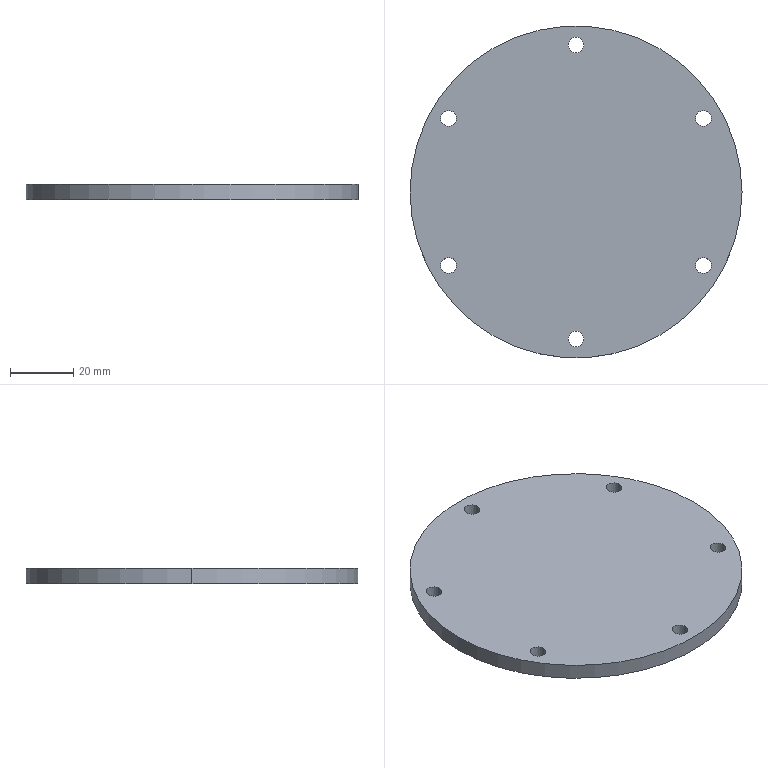Part | STEP file | smoke vent cover plate | 1 solid | 16 faces | box 105 x 105 x 5 mm | volume 42706 mm3 | cylinder 14 | plane 2 | commonest cylinder face diameters 5 x12 105 x2
STEP:
#1=CARTESIAN_POINT('',(0.,0.,0.));
#2=DIRECTION('',(0.,0.,1.));
#3=DIRECTION('',(1.,0.,0.));
#4=AXIS2_PLACEMENT_3D('',#1,#2,#3);
#5=CARTESIAN_POINT('',(-42.77,23.25,5.));
#6=VERTEX_POINT('',#5);
#7=CARTESIAN_POINT('',(-42.77,23.25,0.));
#8=VERTEX_POINT('',#7);
#9=CARTESIAN_POINT('',(-42.77,23.25,5.));
#10=DIRECTION('',(0.,0.,-1.));
#11=VECTOR('',#10,1.);
#12=LINE('',#9,#11);
#13=CARTESIAN_POINT('',(-40.27,23.25,5.));
#14=DIRECTION('',(0.,0.,-1.));
#15=DIRECTION('',(-1.,0.,0.));
#16=AXIS2_PLACEMENT_3D('',#13,#14,#15);
#17=CYLINDRICAL_SURFACE('',#16,2.5);
#18=CARTESIAN_POINT('',(6.283,0.));
#19=DIRECTION('',(0.,1.));
#20=VECTOR('',#19,1.);
#21=LINE('',#18,#20);
#22=(GEOMETRIC_REPRESENTATION_CONTEXT(2)PARAMETRIC_REPRESENTATION_CONTEXT()REPRESENTATION_CONTEXT('',''));
#23=DEFINITIONAL_REPRESENTATION('',(#21),#22);
#24=PCURVE('',#17,#23);
#25=CARTESIAN_POINT('',(-40.27,23.25,5.));
#26=DIRECTION('',(0.,0.,-1.));
#27=DIRECTION('',(-1.,0.,0.));
#28=AXIS2_PLACEMENT_3D('',#25,#26,#27);
#29=CYLINDRICAL_SURFACE('',#28,2.5);
#30=CARTESIAN_POINT('',(0.,0.));
#31=DIRECTION('',(0.,1.));
#32=VECTOR('',#31,1.);
#33=LINE('',#30,#32);
#34=(GEOMETRIC_REPRESENTATION_CONTEXT(2)PARAMETRIC_REPRESENTATION_CONTEXT()REPRESENTATION_CONTEXT('',''));
#35=DEFINITIONAL_REPRESENTATION('',(#33),#34);
#36=PCURVE('',#29,#35);
#37=SURFACE_CURVE('',#12,(#24,#36),.PCURVE_S1.);
#38=EDGE_CURVE('',#6,#8,#37,.T.);
#39=ORIENTED_EDGE('',*,*,#38,.T.);
#40=CARTESIAN_POINT('',(-37.77,23.25,0.));
#41=VERTEX_POINT('',#40);
#42=CARTESIAN_POINT('',(-40.27,23.25,0.));
#43=DIRECTION('',(0.,0.,1.));
#44=DIRECTION('',(1.,0.,0.));
#45=AXIS2_PLACEMENT_3D('',#42,#43,#44);
#46=CIRCLE('',#45,2.5);
#47=CARTESIAN_POINT('',(9.425,5.));
#48=DIRECTION('',(-1.,0.));
#49=VECTOR('',#48,1.);
#50=LINE('',#47,#49);
#51=(GEOMETRIC_REPRESENTATION_CONTEXT(2)PARAMETRIC_REPRESENTATION_CONTEXT()REPRESENTATION_CONTEXT('',''));
#52=DEFINITIONAL_REPRESENTATION('',(#50),#51);
#53=PCURVE('',#17,#52);
#54=CARTESIAN_POINT('',(0.,0.,0.));
#55=DIRECTION('',(0.,0.,1.));
#56=DIRECTION('',(1.,0.,0.));
#57=AXIS2_PLACEMENT_3D('',#54,#55,#56);
#58=PLANE('',#57);
#59=CARTESIAN_POINT('',(-40.27,23.25));
#60=DIRECTION('',(1.,0.));
#61=AXIS2_PLACEMENT_2D('',#59,#60);
#62=CIRCLE('',#61,2.5);
#63=(GEOMETRIC_REPRESENTATION_CONTEXT(2)PARAMETRIC_REPRESENTATION_CONTEXT()REPRESENTATION_CONTEXT('',''));
#64=DEFINITIONAL_REPRESENTATION('',(#62),#63);
#65=PCURVE('',#58,#64);
#66=SURFACE_CURVE('',#46,(#53,#65),.PCURVE_S1.);
#67=EDGE_CURVE('',#8,#41,#66,.T.);
#68=ORIENTED_EDGE('',*,*,#67,.T.);
#69=CARTESIAN_POINT('',(-37.77,23.25,5.));
#70=VERTEX_POINT('',#69);
#71=CARTESIAN_POINT('',(-37.77,23.25,5.));
#72=DIRECTION('',(0.,0.,-1.));
#73=VECTOR('',#72,1.);
#74=LINE('',#71,#73);
#75=CARTESIAN_POINT('',(3.142,0.));
#76=DIRECTION('',(0.,1.));
#77=VECTOR('',#76,1.);
#78=LINE('',#75,#77);
#79=(GEOMETRIC_REPRESENTATION_CONTEXT(2)PARAMETRIC_REPRESENTATION_CONTEXT()REPRESENTATION_CONTEXT('',''));
#80=DEFINITIONAL_REPRESENTATION('',(#78),#79);
#81=PCURVE('',#17,#80);
#82=CARTESIAN_POINT('',(3.142,0.));
#83=DIRECTION('',(0.,1.));
#84=VECTOR('',#83,1.);
#85=LINE('',#82,#84);
#86=(GEOMETRIC_REPRESENTATION_CONTEXT(2)PARAMETRIC_REPRESENTATION_CONTEXT()REPRESENTATION_CONTEXT('',''));
#87=DEFINITIONAL_REPRESENTATION('',(#85),#86);
#88=PCURVE('',#29,#87);
#89=SURFACE_CURVE('',#74,(#81,#88),.PCURVE_S1.);
#90=EDGE_CURVE('',#70,#41,#89,.T.);
#91=ORIENTED_EDGE('',*,*,#90,.F.);
#92=CARTESIAN_POINT('',(-40.27,23.25,5.));
#93=DIRECTION('',(0.,0.,1.));
#94=DIRECTION('',(1.,0.,0.));
#95=AXIS2_PLACEMENT_3D('',#92,#93,#94);
#96=CIRCLE('',#95,2.5);
#97=CARTESIAN_POINT('',(9.425,0.));
#98=DIRECTION('',(-1.,0.));
#99=VECTOR('',#98,1.);
#100=LINE('',#97,#99);
#101=(GEOMETRIC_REPRESENTATION_CONTEXT(2)PARAMETRIC_REPRESENTATION_CONTEXT()REPRESENTATION_CONTEXT('',''));
#102=DEFINITIONAL_REPRESENTATION('',(#100),#101);
#103=PCURVE('',#17,#102);
#104=CARTESIAN_POINT('',(0.,0.,5.));
#105=DIRECTION('',(0.,0.,1.));
#106=DIRECTION('',(1.,0.,0.));
#107=AXIS2_PLACEMENT_3D('',#104,#105,#106);
#108=PLANE('',#107);
#109=CARTESIAN_POINT('',(-40.27,23.25));
#110=DIRECTION('',(1.,0.));
#111=AXIS2_PLACEMENT_2D('',#109,#110);
#112=CIRCLE('',#111,2.5);
#113=(GEOMETRIC_REPRESENTATION_CONTEXT(2)PARAMETRIC_REPRESENTATION_CONTEXT()REPRESENTATION_CONTEXT('',''));
#114=DEFINITIONAL_REPRESENTATION('',(#112),#113);
#115=PCURVE('',#108,#114);
#116=SURFACE_CURVE('',#96,(#103,#115),.PCURVE_S1.);
#117=EDGE_CURVE('',#6,#70,#116,.T.);
#118=ORIENTED_EDGE('',*,*,#117,.F.);
#119=EDGE_LOOP('',(#39,#68,#91,#118));
#120=FACE_BOUND('',#119,.F.);
#121=ADVANCED_FACE('',(#120),#17,.F.);
#122=CARTESIAN_POINT('',(-42.77,-23.25,5.));
#123=VERTEX_POINT('',#122);
#124=CARTESIAN_POINT('',(-42.77,-23.25,0.));
#125=VERTEX_POINT('',#124);
#126=CARTESIAN_POINT('',(-42.77,-23.25,5.));
#127=DIRECTION('',(0.,0.,-1.));
#128=VECTOR('',#127,1.);
#129=LINE('',#126,#128);
#130=CARTESIAN_POINT('',(-40.27,-23.25,5.));
#131=DIRECTION('',(0.,0.,-1.));
#132=DIRECTION('',(-1.,0.,0.));
#133=AXIS2_PLACEMENT_3D('',#130,#131,#132);
#134=CYLINDRICAL_SURFACE('',#133,2.5);
#135=CARTESIAN_POINT('',(6.283,0.));
#136=DIRECTION('',(0.,1.));
#137=VECTOR('',#136,1.);
#138=LINE('',#135,#137);
#139=(GEOMETRIC_REPRESENTATION_CONTEXT(2)PARAMETRIC_REPRESENTATION_CONTEXT()REPRESENTATION_CONTEXT('',''));
#140=DEFINITIONAL_REPRESENTATION('',(#138),#139);
#141=PCURVE('',#134,#140);
#142=CARTESIAN_POINT('',(-40.27,-23.25,5.));
#143=DIRECTION('',(0.,0.,-1.));
#144=DIRECTION('',(-1.,0.,0.));
#145=AXIS2_PLACEMENT_3D('',#142,#143,#144);
#146=CYLINDRICAL_SURFACE('',#145,2.5);
#147=CARTESIAN_POINT('',(0.,0.));
#148=DIRECTION('',(0.,1.));
#149=VECTOR('',#148,1.);
#150=LINE('',#147,#149);
#151=(GEOMETRIC_REPRESENTATION_CONTEXT(2)PARAMETRIC_REPRESENTATION_CONTEXT()REPRESENTATION_CONTEXT('',''));
#152=DEFINITIONAL_REPRESENTATION('',(#150),#151);
#153=PCURVE('',#146,#152);
#154=SURFACE_CURVE('',#129,(#141,#153),.PCURVE_S1.);
#155=EDGE_CURVE('',#123,#125,#154,.T.);
#156=ORIENTED_EDGE('',*,*,#155,.T.);
#157=CARTESIAN_POINT('',(-37.77,-23.25,0.));
#158=VERTEX_POINT('',#157);
#159=CARTESIAN_POINT('',(-40.27,-23.25,0.));
#160=DIRECTION('',(0.,0.,1.));
#161=DIRECTION('',(1.,0.,0.));
#162=AXIS2_PLACEMENT_3D('',#159,#160,#161);
#163=CIRCLE('',#162,2.5);
#164=CARTESIAN_POINT('',(9.425,5.));
#165=DIRECTION('',(-1.,0.));
#166=VECTOR('',#165,1.);
#167=LINE('',#164,#166);
#168=(GEOMETRIC_REPRESENTATION_CONTEXT(2)PARAMETRIC_REPRESENTATION_CONTEXT()REPRESENTATION_CONTEXT('',''));
#169=DEFINITIONAL_REPRESENTATION('',(#167),#168);
#170=PCURVE('',#134,#169);
#171=CARTESIAN_POINT('',(-40.27,-23.25));
#172=DIRECTION('',(1.,0.));
#173=AXIS2_PLACEMENT_2D('',#171,#172);
#174=CIRCLE('',#173,2.5);
#175=(GEOMETRIC_REPRESENTATION_CONTEXT(2)PARAMETRIC_REPRESENTATION_CONTEXT()REPRESENTATION_CONTEXT('',''));
#176=DEFINITIONAL_REPRESENTATION('',(#174),#175);
#177=PCURVE('',#58,#176);
#178=SURFACE_CURVE('',#163,(#170,#177),.PCURVE_S1.);
#179=EDGE_CURVE('',#125,#158,#178,.T.);
#180=ORIENTED_EDGE('',*,*,#179,.T.);
#181=CARTESIAN_POINT('',(-37.77,-23.25,5.));
#182=VERTEX_POINT('',#181);
#183=CARTESIAN_POINT('',(-37.77,-23.25,5.));
#184=DIRECTION('',(0.,0.,-1.));
#185=VECTOR('',#184,1.);
#186=LINE('',#183,#185);
#187=CARTESIAN_POINT('',(3.142,0.));
#188=DIRECTION('',(0.,1.));
#189=VECTOR('',#188,1.);
#190=LINE('',#187,#189);
#191=(GEOMETRIC_REPRESENTATION_CONTEXT(2)PARAMETRIC_REPRESENTATION_CONTEXT()REPRESENTATION_CONTEXT('',''));
#192=DEFINITIONAL_REPRESENTATION('',(#190),#191);
#193=PCURVE('',#134,#192);
#194=CARTESIAN_POINT('',(3.142,0.));
#195=DIRECTION('',(0.,1.));
#196=VECTOR('',#195,1.);
#197=LINE('',#194,#196);
#198=(GEOMETRIC_REPRESENTATION_CONTEXT(2)PARAMETRIC_REPRESENTATION_CONTEXT()REPRESENTATION_CONTEXT('',''));
#199=DEFINITIONAL_REPRESENTATION('',(#197),#198);
#200=PCURVE('',#146,#199);
#201=SURFACE_CURVE('',#186,(#193,#200),.PCURVE_S1.);
#202=EDGE_CURVE('',#182,#158,#201,.T.);
#203=ORIENTED_EDGE('',*,*,#202,.F.);
#204=CARTESIAN_POINT('',(-40.27,-23.25,5.));
#205=DIRECTION('',(0.,0.,1.));
#206=DIRECTION('',(1.,0.,0.));
#207=AXIS2_PLACEMENT_3D('',#204,#205,#206);
#208=CIRCLE('',#207,2.5);
#209=CARTESIAN_POINT('',(9.425,0.));
#210=DIRECTION('',(-1.,0.));
#211=VECTOR('',#210,1.);
#212=LINE('',#209,#211);
#213=(GEOMETRIC_REPRESENTATION_CONTEXT(2)PARAMETRIC_REPRESENTATION_CONTEXT()REPRESENTATION_CONTEXT('',''));
#214=DEFINITIONAL_REPRESENTATION('',(#212),#213);
#215=PCURVE('',#134,#214);
#216=CARTESIAN_POINT('',(-40.27,-23.25));
#217=DIRECTION('',(1.,0.));
#218=AXIS2_PLACEMENT_2D('',#216,#217);
#219=CIRCLE('',#218,2.5);
#220=(GEOMETRIC_REPRESENTATION_CONTEXT(2)PARAMETRIC_REPRESENTATION_CONTEXT()REPRESENTATION_CONTEXT('',''));
#221=DEFINITIONAL_REPRESENTATION('',(#219),#220);
#222=PCURVE('',#108,#221);
#223=SURFACE_CURVE('',#208,(#215,#222),.PCURVE_S1.);
#224=EDGE_CURVE('',#123,#182,#223,.T.);
#225=ORIENTED_EDGE('',*,*,#224,.F.);
#226=EDGE_LOOP('',(#156,#180,#203,#225));
#227=FACE_BOUND('',#226,.F.);
#228=ADVANCED_FACE('',(#227),#134,.F.);
#229=CARTESIAN_POINT('',(-2.5,-46.5,5.));
#230=VERTEX_POINT('',#229);
#231=CARTESIAN_POINT('',(-2.5,-46.5,0.));
#232=VERTEX_POINT('',#231);
#233=CARTESIAN_POINT('',(-2.5,-46.5,5.));
#234=DIRECTION('',(0.,0.,-1.));
#235=VECTOR('',#234,1.);
#236=LINE('',#233,#235);
#237=CARTESIAN_POINT('',(0.,-46.5,5.));
#238=DIRECTION('',(0.,0.,-1.));
#239=DIRECTION('',(-1.,0.,0.));
#240=AXIS2_PLACEMENT_3D('',#237,#238,#239);
#241=CYLINDRICAL_SURFACE('',#240,2.5);
#242=CARTESIAN_POINT('',(6.283,0.));
#243=DIRECTION('',(0.,1.));
#244=VECTOR('',#243,1.);
#245=LINE('',#242,#244);
#246=(GEOMETRIC_REPRESENTATION_CONTEXT(2)PARAMETRIC_REPRESENTATION_CONTEXT()REPRESENTATION_CONTEXT('',''));
#247=DEFINITIONAL_REPRESENTATION('',(#245),#246);
#248=PCURVE('',#241,#247);
#249=CARTESIAN_POINT('',(0.,-46.5,5.));
#250=DIRECTION('',(0.,0.,-1.));
#251=DIRECTION('',(-1.,0.,0.));
#252=AXIS2_PLACEMENT_3D('',#249,#250,#251);
#253=CYLINDRICAL_SURFACE('',#252,2.5);
#254=CARTESIAN_POINT('',(0.,0.));
#255=DIRECTION('',(0.,1.));
#256=VECTOR('',#255,1.);
#257=LINE('',#254,#256);
#258=(GEOMETRIC_REPRESENTATION_CONTEXT(2)PARAMETRIC_REPRESENTATION_CONTEXT()REPRESENTATION_CONTEXT('',''));
#259=DEFINITIONAL_REPRESENTATION('',(#257),#258);
#260=PCURVE('',#253,#259);
#261=SURFACE_CURVE('',#236,(#248,#260),.PCURVE_S1.);
#262=EDGE_CURVE('',#230,#232,#261,.T.);
#263=ORIENTED_EDGE('',*,*,#262,.T.);
#264=CARTESIAN_POINT('',(2.5,-46.5,0.));
#265=VERTEX_POINT('',#264);
#266=CARTESIAN_POINT('',(0.,-46.5,0.));
#267=DIRECTION('',(0.,0.,1.));
#268=DIRECTION('',(1.,0.,0.));
#269=AXIS2_PLACEMENT_3D('',#266,#267,#268);
#270=CIRCLE('',#269,2.5);
#271=CARTESIAN_POINT('',(9.425,5.));
#272=DIRECTION('',(-1.,0.));
#273=VECTOR('',#272,1.);
#274=LINE('',#271,#273);
#275=(GEOMETRIC_REPRESENTATION_CONTEXT(2)PARAMETRIC_REPRESENTATION_CONTEXT()REPRESENTATION_CONTEXT('',''));
#276=DEFINITIONAL_REPRESENTATION('',(#274),#275);
#277=PCURVE('',#241,#276);
#278=CARTESIAN_POINT('',(0.,-46.5));
#279=DIRECTION('',(1.,0.));
#280=AXIS2_PLACEMENT_2D('',#278,#279);
#281=CIRCLE('',#280,2.5);
#282=(GEOMETRIC_REPRESENTATION_CONTEXT(2)PARAMETRIC_REPRESENTATION_CONTEXT()REPRESENTATION_CONTEXT('',''));
#283=DEFINITIONAL_REPRESENTATION('',(#281),#282);
#284=PCURVE('',#58,#283);
#285=SURFACE_CURVE('',#270,(#277,#284),.PCURVE_S1.);
#286=EDGE_CURVE('',#232,#265,#285,.T.);
#287=ORIENTED_EDGE('',*,*,#286,.T.);
#288=CARTESIAN_POINT('',(2.5,-46.5,5.));
#289=VERTEX_POINT('',#288);
#290=CARTESIAN_POINT('',(2.5,-46.5,5.));
#291=DIRECTION('',(0.,0.,-1.));
#292=VECTOR('',#291,1.);
#293=LINE('',#290,#292);
#294=CARTESIAN_POINT('',(3.142,0.));
#295=DIRECTION('',(0.,1.));
#296=VECTOR('',#295,1.);
#297=LINE('',#294,#296);
#298=(GEOMETRIC_REPRESENTATION_CONTEXT(2)PARAMETRIC_REPRESENTATION_CONTEXT()REPRESENTATION_CONTEXT('',''));
#299=DEFINITIONAL_REPRESENTATION('',(#297),#298);
#300=PCURVE('',#241,#299);
#301=CARTESIAN_POINT('',(3.142,0.));
#302=DIRECTION('',(0.,1.));
#303=VECTOR('',#302,1.);
#304=LINE('',#301,#303);
#305=(GEOMETRIC_REPRESENTATION_CONTEXT(2)PARAMETRIC_REPRESENTATION_CONTEXT()REPRESENTATION_CONTEXT('',''));
#306=DEFINITIONAL_REPRESENTATION('',(#304),#305);
#307=PCURVE('',#253,#306);
#308=SURFACE_CURVE('',#293,(#300,#307),.PCURVE_S1.);
#309=EDGE_CURVE('',#289,#265,#308,.T.);
#310=ORIENTED_EDGE('',*,*,#309,.F.);
#311=CARTESIAN_POINT('',(0.,-46.5,5.));
#312=DIRECTION('',(0.,0.,1.));
#313=DIRECTION('',(1.,0.,0.));
#314=AXIS2_PLACEMENT_3D('',#311,#312,#313);
#315=CIRCLE('',#314,2.5);
#316=CARTESIAN_POINT('',(9.425,0.));
#317=DIRECTION('',(-1.,0.));
#318=VECTOR('',#317,1.);
#319=LINE('',#316,#318);
#320=(GEOMETRIC_REPRESENTATION_CONTEXT(2)PARAMETRIC_REPRESENTATION_CONTEXT()REPRESENTATION_CONTEXT('',''));
#321=DEFINITIONAL_REPRESENTATION('',(#319),#320);
#322=PCURVE('',#241,#321);
#323=CARTESIAN_POINT('',(0.,-46.5));
#324=DIRECTION('',(1.,0.));
#325=AXIS2_PLACEMENT_2D('',#323,#324);
#326=CIRCLE('',#325,2.5);
#327=(GEOMETRIC_REPRESENTATION_CONTEXT(2)PARAMETRIC_REPRESENTATION_CONTEXT()REPRESENTATION_CONTEXT('',''));
#328=DEFINITIONAL_REPRESENTATION('',(#326),#327);
#329=PCURVE('',#108,#328);
#330=SURFACE_CURVE('',#315,(#322,#329),.PCURVE_S1.);
#331=EDGE_CURVE('',#230,#289,#330,.T.);
#332=ORIENTED_EDGE('',*,*,#331,.F.);
#333=EDGE_LOOP('',(#263,#287,#310,#332));
#334=FACE_BOUND('',#333,.F.);
#335=ADVANCED_FACE('',(#334),#241,.F.);
#336=CARTESIAN_POINT('',(37.77,-23.25,5.));
#337=VERTEX_POINT('',#336);
#338=CARTESIAN_POINT('',(37.77,-23.25,0.));
#339=VERTEX_POINT('',#338);
#340=CARTESIAN_POINT('',(37.77,-23.25,5.));
#341=DIRECTION('',(0.,0.,-1.));
#342=VECTOR('',#341,1.);
#343=LINE('',#340,#342);
#344=CARTESIAN_POINT('',(40.27,-23.25,5.));
#345=DIRECTION('',(0.,0.,-1.));
#346=DIRECTION('',(-1.,0.,0.));
#347=AXIS2_PLACEMENT_3D('',#344,#345,#346);
#348=CYLINDRICAL_SURFACE('',#347,2.5);
#349=CARTESIAN_POINT('',(6.283,0.));
#350=DIRECTION('',(0.,1.));
#351=VECTOR('',#350,1.);
#352=LINE('',#349,#351);
#353=(GEOMETRIC_REPRESENTATION_CONTEXT(2)PARAMETRIC_REPRESENTATION_CONTEXT()REPRESENTATION_CONTEXT('',''));
#354=DEFINITIONAL_REPRESENTATION('',(#352),#353);
#355=PCURVE('',#348,#354);
#356=CARTESIAN_POINT('',(40.27,-23.25,5.));
#357=DIRECTION('',(0.,0.,-1.));
#358=DIRECTION('',(-1.,0.,0.));
#359=AXIS2_PLACEMENT_3D('',#356,#357,#358);
#360=CYLINDRICAL_SURFACE('',#359,2.5);
#361=CARTESIAN_POINT('',(0.,0.));
#362=DIRECTION('',(0.,1.));
#363=VECTOR('',#362,1.);
#364=LINE('',#361,#363);
#365=(GEOMETRIC_REPRESENTATION_CONTEXT(2)PARAMETRIC_REPRESENTATION_CONTEXT()REPRESENTATION_CONTEXT('',''));
#366=DEFINITIONAL_REPRESENTATION('',(#364),#365);
#367=PCURVE('',#360,#366);
#368=SURFACE_CURVE('',#343,(#355,#367),.PCURVE_S1.);
#369=EDGE_CURVE('',#337,#339,#368,.T.);
#370=ORIENTED_EDGE('',*,*,#369,.T.);
#371=CARTESIAN_POINT('',(42.77,-23.25,0.));
#372=VERTEX_POINT('',#371);
#373=CARTESIAN_POINT('',(40.27,-23.25,0.));
#374=DIRECTION('',(0.,0.,1.));
#375=DIRECTION('',(1.,0.,0.));
#376=AXIS2_PLACEMENT_3D('',#373,#374,#375);
#377=CIRCLE('',#376,2.5);
#378=CARTESIAN_POINT('',(9.425,5.));
#379=DIRECTION('',(-1.,0.));
#380=VECTOR('',#379,1.);
#381=LINE('',#378,#380);
#382=(GEOMETRIC_REPRESENTATION_CONTEXT(2)PARAMETRIC_REPRESENTATION_CONTEXT()REPRESENTATION_CONTEXT('',''));
#383=DEFINITIONAL_REPRESENTATION('',(#381),#382);
#384=PCURVE('',#348,#383);
#385=CARTESIAN_POINT('',(40.27,-23.25));
#386=DIRECTION('',(1.,0.));
#387=AXIS2_PLACEMENT_2D('',#385,#386);
#388=CIRCLE('',#387,2.5);
#389=(GEOMETRIC_REPRESENTATION_CONTEXT(2)PARAMETRIC_REPRESENTATION_CONTEXT()REPRESENTATION_CONTEXT('',''));
#390=DEFINITIONAL_REPRESENTATION('',(#388),#389);
#391=PCURVE('',#58,#390);
#392=SURFACE_CURVE('',#377,(#384,#391),.PCURVE_S1.);
#393=EDGE_CURVE('',#339,#372,#392,.T.);
#394=ORIENTED_EDGE('',*,*,#393,.T.);
#395=CARTESIAN_POINT('',(42.77,-23.25,5.));
#396=VERTEX_POINT('',#395);
#397=CARTESIAN_POINT('',(42.77,-23.25,5.));
#398=DIRECTION('',(0.,0.,-1.));
#399=VECTOR('',#398,1.);
#400=LINE('',#397,#399);
#401=CARTESIAN_POINT('',(3.142,0.));
#402=DIRECTION('',(0.,1.));
#403=VECTOR('',#402,1.);
#404=LINE('',#401,#403);
#405=(GEOMETRIC_REPRESENTATION_CONTEXT(2)PARAMETRIC_REPRESENTATION_CONTEXT()REPRESENTATION_CONTEXT('',''));
#406=DEFINITIONAL_REPRESENTATION('',(#404),#405);
#407=PCURVE('',#348,#406);
#408=CARTESIAN_POINT('',(3.142,0.));
#409=DIRECTION('',(0.,1.));
#410=VECTOR('',#409,1.);
#411=LINE('',#408,#410);
#412=(GEOMETRIC_REPRESENTATION_CONTEXT(2)PARAMETRIC_REPRESENTATION_CONTEXT()REPRESENTATION_CONTEXT('',''));
#413=DEFINITIONAL_REPRESENTATION('',(#411),#412);
#414=PCURVE('',#360,#413);
#415=SURFACE_CURVE('',#400,(#407,#414),.PCURVE_S1.);
#416=EDGE_CURVE('',#396,#372,#415,.T.);
#417=ORIENTED_EDGE('',*,*,#416,.F.);
#418=CARTESIAN_POINT('',(40.27,-23.25,5.));
#419=DIRECTION('',(0.,0.,1.));
#420=DIRECTION('',(1.,0.,0.));
#421=AXIS2_PLACEMENT_3D('',#418,#419,#420);
#422=CIRCLE('',#421,2.5);
#423=CARTESIAN_POINT('',(9.425,0.));
#424=DIRECTION('',(-1.,0.));
#425=VECTOR('',#424,1.);
#426=LINE('',#423,#425);
#427=(GEOMETRIC_REPRESENTATION_CONTEXT(2)PARAMETRIC_REPRESENTATION_CONTEXT()REPRESENTATION_CONTEXT('',''));
#428=DEFINITIONAL_REPRESENTATION('',(#426),#427);
#429=PCURVE('',#348,#428);
#430=CARTESIAN_POINT('',(40.27,-23.25));
#431=DIRECTION('',(1.,0.));
#432=AXIS2_PLACEMENT_2D('',#430,#431);
#433=CIRCLE('',#432,2.5);
#434=(GEOMETRIC_REPRESENTATION_CONTEXT(2)PARAMETRIC_REPRESENTATION_CONTEXT()REPRESENTATION_CONTEXT('',''));
#435=DEFINITIONAL_REPRESENTATION('',(#433),#434);
#436=PCURVE('',#108,#435);
#437=SURFACE_CURVE('',#422,(#429,#436),.PCURVE_S1.);
#438=EDGE_CURVE('',#337,#396,#437,.T.);
#439=ORIENTED_EDGE('',*,*,#438,.F.);
#440=EDGE_LOOP('',(#370,#394,#417,#439));
#441=FACE_BOUND('',#440,.F.);
#442=ADVANCED_FACE('',(#441),#348,.F.);
#443=CARTESIAN_POINT('',(37.77,23.25,5.));
#444=VERTEX_POINT('',#443);
#445=CARTESIAN_POINT('',(37.77,23.25,0.));
#446=VERTEX_POINT('',#445);
#447=CARTESIAN_POINT('',(37.77,23.25,5.));
#448=DIRECTION('',(0.,0.,-1.));
#449=VECTOR('',#448,1.);
#450=LINE('',#447,#449);
#451=CARTESIAN_POINT('',(40.27,23.25,5.));
#452=DIRECTION('',(0.,0.,-1.));
#453=DIRECTION('',(-1.,0.,0.));
#454=AXIS2_PLACEMENT_3D('',#451,#452,#453);
#455=CYLINDRICAL_SURFACE('',#454,2.5);
#456=CARTESIAN_POINT('',(6.283,0.));
#457=DIRECTION('',(0.,1.));
#458=VECTOR('',#457,1.);
#459=LINE('',#456,#458);
#460=(GEOMETRIC_REPRESENTATION_CONTEXT(2)PARAMETRIC_REPRESENTATION_CONTEXT()REPRESENTATION_CONTEXT('',''));
#461=DEFINITIONAL_REPRESENTATION('',(#459),#460);
#462=PCURVE('',#455,#461);
#463=CARTESIAN_POINT('',(40.27,23.25,5.));
#464=DIRECTION('',(0.,0.,-1.));
#465=DIRECTION('',(-1.,0.,0.));
#466=AXIS2_PLACEMENT_3D('',#463,#464,#465);
#467=CYLINDRICAL_SURFACE('',#466,2.5);
#468=CARTESIAN_POINT('',(0.,0.));
#469=DIRECTION('',(0.,1.));
#470=VECTOR('',#469,1.);
#471=LINE('',#468,#470);
#472=(GEOMETRIC_REPRESENTATION_CONTEXT(2)PARAMETRIC_REPRESENTATION_CONTEXT()REPRESENTATION_CONTEXT('',''));
#473=DEFINITIONAL_REPRESENTATION('',(#471),#472);
#474=PCURVE('',#467,#473);
#475=SURFACE_CURVE('',#450,(#462,#474),.PCURVE_S1.);
#476=EDGE_CURVE('',#444,#446,#475,.T.);
#477=ORIENTED_EDGE('',*,*,#476,.T.);
#478=CARTESIAN_POINT('',(42.77,23.25,0.));
#479=VERTEX_POINT('',#478);
#480=CARTESIAN_POINT('',(40.27,23.25,0.));
#481=DIRECTION('',(0.,0.,1.));
#482=DIRECTION('',(1.,0.,0.));
#483=AXIS2_PLACEMENT_3D('',#480,#481,#482);
#484=CIRCLE('',#483,2.5);
#485=CARTESIAN_POINT('',(9.425,5.));
#486=DIRECTION('',(-1.,0.));
#487=VECTOR('',#486,1.);
#488=LINE('',#485,#487);
#489=(GEOMETRIC_REPRESENTATION_CONTEXT(2)PARAMETRIC_REPRESENTATION_CONTEXT()REPRESENTATION_CONTEXT('',''));
#490=DEFINITIONAL_REPRESENTATION('',(#488),#489);
#491=PCURVE('',#455,#490);
#492=CARTESIAN_POINT('',(40.27,23.25));
#493=DIRECTION('',(1.,0.));
#494=AXIS2_PLACEMENT_2D('',#492,#493);
#495=CIRCLE('',#494,2.5);
#496=(GEOMETRIC_REPRESENTATION_CONTEXT(2)PARAMETRIC_REPRESENTATION_CONTEXT()REPRESENTATION_CONTEXT('',''));
#497=DEFINITIONAL_REPRESENTATION('',(#495),#496);
#498=PCURVE('',#58,#497);
#499=SURFACE_CURVE('',#484,(#491,#498),.PCURVE_S1.);
#500=EDGE_CURVE('',#446,#479,#499,.T.);
#501=ORIENTED_EDGE('',*,*,#500,.T.);
#502=CARTESIAN_POINT('',(42.77,23.25,5.));
#503=VERTEX_POINT('',#502);
#504=CARTESIAN_POINT('',(42.77,23.25,5.));
#505=DIRECTION('',(0.,0.,-1.));
#506=VECTOR('',#505,1.);
#507=LINE('',#504,#506);
#508=CARTESIAN_POINT('',(3.142,0.));
#509=DIRECTION('',(0.,1.));
#510=VECTOR('',#509,1.);
#511=LINE('',#508,#510);
#512=(GEOMETRIC_REPRESENTATION_CONTEXT(2)PARAMETRIC_REPRESENTATION_CONTEXT()REPRESENTATION_CONTEXT('',''));
#513=DEFINITIONAL_REPRESENTATION('',(#511),#512);
#514=PCURVE('',#455,#513);
#515=CARTESIAN_POINT('',(3.142,0.));
#516=DIRECTION('',(0.,1.));
#517=VECTOR('',#516,1.);
#518=LINE('',#515,#517);
#519=(GEOMETRIC_REPRESENTATION_CONTEXT(2)PARAMETRIC_REPRESENTATION_CONTEXT()REPRESENTATION_CONTEXT('',''));
#520=DEFINITIONAL_REPRESENTATION('',(#518),#519);
#521=PCURVE('',#467,#520);
#522=SURFACE_CURVE('',#507,(#514,#521),.PCURVE_S1.);
#523=EDGE_CURVE('',#503,#479,#522,.T.);
#524=ORIENTED_EDGE('',*,*,#523,.F.);
#525=CARTESIAN_POINT('',(40.27,23.25,5.));
#526=DIRECTION('',(0.,0.,1.));
#527=DIRECTION('',(1.,0.,0.));
#528=AXIS2_PLACEMENT_3D('',#525,#526,#527);
#529=CIRCLE('',#528,2.5);
#530=CARTESIAN_POINT('',(9.425,0.));
#531=DIRECTION('',(-1.,0.));
#532=VECTOR('',#531,1.);
#533=LINE('',#530,#532);
#534=(GEOMETRIC_REPRESENTATION_CONTEXT(2)PARAMETRIC_REPRESENTATION_CONTEXT()REPRESENTATION_CONTEXT('',''));
#535=DEFINITIONAL_REPRESENTATION('',(#533),#534);
#536=PCURVE('',#455,#535);
#537=CARTESIAN_POINT('',(40.27,23.25));
#538=DIRECTION('',(1.,0.));
#539=AXIS2_PLACEMENT_2D('',#537,#538);
#540=CIRCLE('',#539,2.5);
#541=(GEOMETRIC_REPRESENTATION_CONTEXT(2)PARAMETRIC_REPRESENTATION_CONTEXT()REPRESENTATION_CONTEXT('',''));
#542=DEFINITIONAL_REPRESENTATION('',(#540),#541);
#543=PCURVE('',#108,#542);
#544=SURFACE_CURVE('',#529,(#536,#543),.PCURVE_S1.);
#545=EDGE_CURVE('',#444,#503,#544,.T.);
#546=ORIENTED_EDGE('',*,*,#545,.F.);
#547=EDGE_LOOP('',(#477,#501,#524,#546));
#548=FACE_BOUND('',#547,.F.);
#549=ADVANCED_FACE('',(#548),#455,.F.);
#550=CARTESIAN_POINT('',(-2.5,46.5,5.));
#551=VERTEX_POINT('',#550);
#552=CARTESIAN_POINT('',(-2.5,46.5,0.));
#553=VERTEX_POINT('',#552);
#554=CARTESIAN_POINT('',(-2.5,46.5,5.));
#555=DIRECTION('',(0.,0.,-1.));
#556=VECTOR('',#555,1.);
#557=LINE('',#554,#556);
#558=CARTESIAN_POINT('',(0.,46.5,5.));
#559=DIRECTION('',(0.,0.,-1.));
#560=DIRECTION('',(-1.,0.,0.));
#561=AXIS2_PLACEMENT_3D('',#558,#559,#560);
#562=CYLINDRICAL_SURFACE('',#561,2.5);
#563=CARTESIAN_POINT('',(6.283,0.));
#564=DIRECTION('',(0.,1.));
#565=VECTOR('',#564,1.);
#566=LINE('',#563,#565);
#567=(GEOMETRIC_REPRESENTATION_CONTEXT(2)PARAMETRIC_REPRESENTATION_CONTEXT()REPRESENTATION_CONTEXT('',''));
#568=DEFINITIONAL_REPRESENTATION('',(#566),#567);
#569=PCURVE('',#562,#568);
#570=CARTESIAN_POINT('',(0.,46.5,5.));
#571=DIRECTION('',(0.,0.,-1.));
#572=DIRECTION('',(-1.,0.,0.));
#573=AXIS2_PLACEMENT_3D('',#570,#571,#572);
#574=CYLINDRICAL_SURFACE('',#573,2.5);
#575=CARTESIAN_POINT('',(0.,0.));
#576=DIRECTION('',(0.,1.));
#577=VECTOR('',#576,1.);
#578=LINE('',#575,#577);
#579=(GEOMETRIC_REPRESENTATION_CONTEXT(2)PARAMETRIC_REPRESENTATION_CONTEXT()REPRESENTATION_CONTEXT('',''));
#580=DEFINITIONAL_REPRESENTATION('',(#578),#579);
#581=PCURVE('',#574,#580);
#582=SURFACE_CURVE('',#557,(#569,#581),.PCURVE_S1.);
#583=EDGE_CURVE('',#551,#553,#582,.T.);
#584=ORIENTED_EDGE('',*,*,#583,.T.);
#585=CARTESIAN_POINT('',(2.5,46.5,0.));
#586=VERTEX_POINT('',#585);
#587=CARTESIAN_POINT('',(0.,46.5,0.));
#588=DIRECTION('',(0.,0.,1.));
#589=DIRECTION('',(1.,0.,0.));
#590=AXIS2_PLACEMENT_3D('',#587,#588,#589);
#591=CIRCLE('',#590,2.5);
#592=CARTESIAN_POINT('',(9.425,5.));
#593=DIRECTION('',(-1.,0.));
#594=VECTOR('',#593,1.);
#595=LINE('',#592,#594);
#596=(GEOMETRIC_REPRESENTATION_CONTEXT(2)PARAMETRIC_REPRESENTATION_CONTEXT()REPRESENTATION_CONTEXT('',''));
#597=DEFINITIONAL_REPRESENTATION('',(#595),#596);
#598=PCURVE('',#562,#597);
#599=CARTESIAN_POINT('',(0.,46.5));
#600=DIRECTION('',(1.,0.));
#601=AXIS2_PLACEMENT_2D('',#599,#600);
#602=CIRCLE('',#601,2.5);
#603=(GEOMETRIC_REPRESENTATION_CONTEXT(2)PARAMETRIC_REPRESENTATION_CONTEXT()REPRESENTATION_CONTEXT('',''));
#604=DEFINITIONAL_REPRESENTATION('',(#602),#603);
#605=PCURVE('',#58,#604);
#606=SURFACE_CURVE('',#591,(#598,#605),.PCURVE_S1.);
#607=EDGE_CURVE('',#553,#586,#606,.T.);
#608=ORIENTED_EDGE('',*,*,#607,.T.);
#609=CARTESIAN_POINT('',(2.5,46.5,5.));
#610=VERTEX_POINT('',#609);
#611=CARTESIAN_POINT('',(2.5,46.5,5.));
#612=DIRECTION('',(0.,0.,-1.));
#613=VECTOR('',#612,1.);
#614=LINE('',#611,#613);
#615=CARTESIAN_POINT('',(3.142,0.));
#616=DIRECTION('',(0.,1.));
#617=VECTOR('',#616,1.);
#618=LINE('',#615,#617);
#619=(GEOMETRIC_REPRESENTATION_CONTEXT(2)PARAMETRIC_REPRESENTATION_CONTEXT()REPRESENTATION_CONTEXT('',''));
#620=DEFINITIONAL_REPRESENTATION('',(#618),#619);
#621=PCURVE('',#562,#620);
#622=CARTESIAN_POINT('',(3.142,0.));
#623=DIRECTION('',(0.,1.));
#624=VECTOR('',#623,1.);
#625=LINE('',#622,#624);
#626=(GEOMETRIC_REPRESENTATION_CONTEXT(2)PARAMETRIC_REPRESENTATION_CONTEXT()REPRESENTATION_CONTEXT('',''));
#627=DEFINITIONAL_REPRESENTATION('',(#625),#626);
#628=PCURVE('',#574,#627);
#629=SURFACE_CURVE('',#614,(#621,#628),.PCURVE_S1.);
#630=EDGE_CURVE('',#610,#586,#629,.T.);
#631=ORIENTED_EDGE('',*,*,#630,.F.);
#632=CARTESIAN_POINT('',(0.,46.5,5.));
#633=DIRECTION('',(0.,0.,1.));
#634=DIRECTION('',(1.,0.,0.));
#635=AXIS2_PLACEMENT_3D('',#632,#633,#634);
#636=CIRCLE('',#635,2.5);
#637=CARTESIAN_POINT('',(9.425,0.));
#638=DIRECTION('',(-1.,0.));
#639=VECTOR('',#638,1.);
#640=LINE('',#637,#639);
#641=(GEOMETRIC_REPRESENTATION_CONTEXT(2)PARAMETRIC_REPRESENTATION_CONTEXT()REPRESENTATION_CONTEXT('',''));
#642=DEFINITIONAL_REPRESENTATION('',(#640),#641);
#643=PCURVE('',#562,#642);
#644=CARTESIAN_POINT('',(0.,46.5));
#645=DIRECTION('',(1.,0.));
#646=AXIS2_PLACEMENT_2D('',#644,#645);
#647=CIRCLE('',#646,2.5);
#648=(GEOMETRIC_REPRESENTATION_CONTEXT(2)PARAMETRIC_REPRESENTATION_CONTEXT()REPRESENTATION_CONTEXT('',''));
#649=DEFINITIONAL_REPRESENTATION('',(#647),#648);
#650=PCURVE('',#108,#649);
#651=SURFACE_CURVE('',#636,(#643,#650),.PCURVE_S1.);
#652=EDGE_CURVE('',#551,#610,#651,.T.);
#653=ORIENTED_EDGE('',*,*,#652,.F.);
#654=EDGE_LOOP('',(#584,#608,#631,#653));
#655=FACE_BOUND('',#654,.F.);
#656=ADVANCED_FACE('',(#655),#562,.F.);
#657=CARTESIAN_POINT('',(52.5,0.,5.));
#658=VERTEX_POINT('',#657);
#659=CARTESIAN_POINT('',(-52.5,0.,5.));
#660=VERTEX_POINT('',#659);
#661=CARTESIAN_POINT('',(0.,0.,5.));
#662=DIRECTION('',(0.,0.,1.));
#663=DIRECTION('',(1.,0.,0.));
#664=AXIS2_PLACEMENT_3D('',#661,#662,#663);
#665=CIRCLE('',#664,52.5);
#666=CARTESIAN_POINT('',(0.,0.,5.));
#667=DIRECTION('',(0.,0.,-1.));
#668=DIRECTION('',(-1.,0.,0.));
#669=AXIS2_PLACEMENT_3D('',#666,#667,#668);
#670=CYLINDRICAL_SURFACE('',#669,52.5);
#671=CARTESIAN_POINT('',(3.142,0.));
#672=DIRECTION('',(-1.,0.));
#673=VECTOR('',#672,1.);
#674=LINE('',#671,#673);
#675=(GEOMETRIC_REPRESENTATION_CONTEXT(2)PARAMETRIC_REPRESENTATION_CONTEXT()REPRESENTATION_CONTEXT('',''));
#676=DEFINITIONAL_REPRESENTATION('',(#674),#675);
#677=PCURVE('',#670,#676);
#678=CARTESIAN_POINT('',(0.,0.));
#679=DIRECTION('',(1.,0.));
#680=AXIS2_PLACEMENT_2D('',#678,#679);
#681=CIRCLE('',#680,52.5);
#682=(GEOMETRIC_REPRESENTATION_CONTEXT(2)PARAMETRIC_REPRESENTATION_CONTEXT()REPRESENTATION_CONTEXT('',''));
#683=DEFINITIONAL_REPRESENTATION('',(#681),#682);
#684=PCURVE('',#108,#683);
#685=SURFACE_CURVE('',#665,(#677,#684),.PCURVE_S1.);
#686=EDGE_CURVE('',#658,#660,#685,.T.);
#687=ORIENTED_EDGE('',*,*,#686,.F.);
#688=CARTESIAN_POINT('',(52.5,0.,0.));
#689=VERTEX_POINT('',#688);
#690=CARTESIAN_POINT('',(52.5,0.,5.));
#691=DIRECTION('',(0.,0.,-1.));
#692=VECTOR('',#691,1.);
#693=LINE('',#690,#692);
#694=CARTESIAN_POINT('',(3.142,0.));
#695=DIRECTION('',(0.,1.));
#696=VECTOR('',#695,1.);
#697=LINE('',#694,#696);
#698=(GEOMETRIC_REPRESENTATION_CONTEXT(2)PARAMETRIC_REPRESENTATION_CONTEXT()REPRESENTATION_CONTEXT('',''));
#699=DEFINITIONAL_REPRESENTATION('',(#697),#698);
#700=PCURVE('',#670,#699);
#701=CARTESIAN_POINT('',(0.,0.,5.));
#702=DIRECTION('',(0.,0.,-1.));
#703=DIRECTION('',(-1.,0.,0.));
#704=AXIS2_PLACEMENT_3D('',#701,#702,#703);
#705=CYLINDRICAL_SURFACE('',#704,52.5);
#706=CARTESIAN_POINT('',(3.142,0.));
#707=DIRECTION('',(0.,1.));
#708=VECTOR('',#707,1.);
#709=LINE('',#706,#708);
#710=(GEOMETRIC_REPRESENTATION_CONTEXT(2)PARAMETRIC_REPRESENTATION_CONTEXT()REPRESENTATION_CONTEXT('',''));
#711=DEFINITIONAL_REPRESENTATION('',(#709),#710);
#712=PCURVE('',#705,#711);
#713=SURFACE_CURVE('',#693,(#700,#712),.PCURVE_S1.);
#714=EDGE_CURVE('',#658,#689,#713,.T.);
#715=ORIENTED_EDGE('',*,*,#714,.T.);
#716=CARTESIAN_POINT('',(-52.5,0.,0.));
#717=VERTEX_POINT('',#716);
#718=CARTESIAN_POINT('',(0.,0.,0.));
#719=DIRECTION('',(0.,0.,1.));
#720=DIRECTION('',(1.,0.,0.));
#721=AXIS2_PLACEMENT_3D('',#718,#719,#720);
#722=CIRCLE('',#721,52.5);
#723=CARTESIAN_POINT('',(3.142,5.));
#724=DIRECTION('',(-1.,0.));
#725=VECTOR('',#724,1.);
#726=LINE('',#723,#725);
#727=(GEOMETRIC_REPRESENTATION_CONTEXT(2)PARAMETRIC_REPRESENTATION_CONTEXT()REPRESENTATION_CONTEXT('',''));
#728=DEFINITIONAL_REPRESENTATION('',(#726),#727);
#729=PCURVE('',#670,#728);
#730=CARTESIAN_POINT('',(0.,0.));
#731=DIRECTION('',(1.,0.));
#732=AXIS2_PLACEMENT_2D('',#730,#731);
#733=CIRCLE('',#732,52.5);
#734=(GEOMETRIC_REPRESENTATION_CONTEXT(2)PARAMETRIC_REPRESENTATION_CONTEXT()REPRESENTATION_CONTEXT('',''));
#735=DEFINITIONAL_REPRESENTATION('',(#733),#734);
#736=PCURVE('',#58,#735);
#737=SURFACE_CURVE('',#722,(#729,#736),.PCURVE_S1.);
#738=EDGE_CURVE('',#689,#717,#737,.T.);
#739=ORIENTED_EDGE('',*,*,#738,.T.);
#740=CARTESIAN_POINT('',(-52.5,0.,5.));
#741=DIRECTION('',(0.,0.,-1.));
#742=VECTOR('',#741,1.);
#743=LINE('',#740,#742);
#744=CARTESIAN_POINT('',(0.,0.));
#745=DIRECTION('',(0.,1.));
#746=VECTOR('',#745,1.);
#747=LINE('',#744,#746);
#748=(GEOMETRIC_REPRESENTATION_CONTEXT(2)PARAMETRIC_REPRESENTATION_CONTEXT()REPRESENTATION_CONTEXT('',''));
#749=DEFINITIONAL_REPRESENTATION('',(#747),#748);
#750=PCURVE('',#670,#749);
#751=CARTESIAN_POINT('',(6.283,0.));
#752=DIRECTION('',(0.,1.));
#753=VECTOR('',#752,1.);
#754=LINE('',#751,#753);
#755=(GEOMETRIC_REPRESENTATION_CONTEXT(2)PARAMETRIC_REPRESENTATION_CONTEXT()REPRESENTATION_CONTEXT('',''));
#756=DEFINITIONAL_REPRESENTATION('',(#754),#755);
#757=PCURVE('',#705,#756);
#758=SURFACE_CURVE('',#743,(#750,#757),.PCURVE_S1.);
#759=EDGE_CURVE('',#660,#717,#758,.T.);
#760=ORIENTED_EDGE('',*,*,#759,.F.);
#761=EDGE_LOOP('',(#687,#715,#739,#760));
#762=FACE_BOUND('',#761,.T.);
#763=ADVANCED_FACE('',(#762),#670,.T.);
#764=ORIENTED_EDGE('',*,*,#224,.F.);
#765=CARTESIAN_POINT('',(-40.27,-23.25,5.));
#766=DIRECTION('',(0.,0.,1.));
#767=DIRECTION('',(1.,0.,0.));
#768=AXIS2_PLACEMENT_3D('',#765,#766,#767);
#769=CIRCLE('',#768,2.5);
#770=CARTESIAN_POINT('',(-40.27,-23.25));
#771=DIRECTION('',(1.,0.));
#772=AXIS2_PLACEMENT_2D('',#770,#771);
#773=CIRCLE('',#772,2.5);
#774=(GEOMETRIC_REPRESENTATION_CONTEXT(2)PARAMETRIC_REPRESENTATION_CONTEXT()REPRESENTATION_CONTEXT('',''));
#775=DEFINITIONAL_REPRESENTATION('',(#773),#774);
#776=PCURVE('',#108,#775);
#777=CARTESIAN_POINT('',(3.142,0.));
#778=DIRECTION('',(-1.,0.));
#779=VECTOR('',#778,1.);
#780=LINE('',#777,#779);
#781=(GEOMETRIC_REPRESENTATION_CONTEXT(2)PARAMETRIC_REPRESENTATION_CONTEXT()REPRESENTATION_CONTEXT('',''));
#782=DEFINITIONAL_REPRESENTATION('',(#780),#781);
#783=PCURVE('',#146,#782);
#784=SURFACE_CURVE('',#769,(#776,#783),.PCURVE_S1.);
#785=EDGE_CURVE('',#182,#123,#784,.T.);
#786=ORIENTED_EDGE('',*,*,#785,.F.);
#787=EDGE_LOOP('',(#764,#786));
#788=FACE_BOUND('',#787,.T.);
#789=ORIENTED_EDGE('',*,*,#438,.F.);
#790=CARTESIAN_POINT('',(40.27,-23.25,5.));
#791=DIRECTION('',(0.,0.,1.));
#792=DIRECTION('',(1.,0.,0.));
#793=AXIS2_PLACEMENT_3D('',#790,#791,#792);
#794=CIRCLE('',#793,2.5);
#795=CARTESIAN_POINT('',(40.27,-23.25));
#796=DIRECTION('',(1.,0.));
#797=AXIS2_PLACEMENT_2D('',#795,#796);
#798=CIRCLE('',#797,2.5);
#799=(GEOMETRIC_REPRESENTATION_CONTEXT(2)PARAMETRIC_REPRESENTATION_CONTEXT()REPRESENTATION_CONTEXT('',''));
#800=DEFINITIONAL_REPRESENTATION('',(#798),#799);
#801=PCURVE('',#108,#800);
#802=CARTESIAN_POINT('',(3.142,0.));
#803=DIRECTION('',(-1.,0.));
#804=VECTOR('',#803,1.);
#805=LINE('',#802,#804);
#806=(GEOMETRIC_REPRESENTATION_CONTEXT(2)PARAMETRIC_REPRESENTATION_CONTEXT()REPRESENTATION_CONTEXT('',''));
#807=DEFINITIONAL_REPRESENTATION('',(#805),#806);
#808=PCURVE('',#360,#807);
#809=SURFACE_CURVE('',#794,(#801,#808),.PCURVE_S1.);
#810=EDGE_CURVE('',#396,#337,#809,.T.);
#811=ORIENTED_EDGE('',*,*,#810,.F.);
#812=EDGE_LOOP('',(#789,#811));
#813=FACE_BOUND('',#812,.T.);
#814=ORIENTED_EDGE('',*,*,#652,.F.);
#815=CARTESIAN_POINT('',(0.,46.5,5.));
#816=DIRECTION('',(0.,0.,1.));
#817=DIRECTION('',(1.,0.,0.));
#818=AXIS2_PLACEMENT_3D('',#815,#816,#817);
#819=CIRCLE('',#818,2.5);
#820=CARTESIAN_POINT('',(0.,46.5));
#821=DIRECTION('',(1.,0.));
#822=AXIS2_PLACEMENT_2D('',#820,#821);
#823=CIRCLE('',#822,2.5);
#824=(GEOMETRIC_REPRESENTATION_CONTEXT(2)PARAMETRIC_REPRESENTATION_CONTEXT()REPRESENTATION_CONTEXT('',''));
#825=DEFINITIONAL_REPRESENTATION('',(#823),#824);
#826=PCURVE('',#108,#825);
#827=CARTESIAN_POINT('',(3.142,0.));
#828=DIRECTION('',(-1.,0.));
#829=VECTOR('',#828,1.);
#830=LINE('',#827,#829);
#831=(GEOMETRIC_REPRESENTATION_CONTEXT(2)PARAMETRIC_REPRESENTATION_CONTEXT()REPRESENTATION_CONTEXT('',''));
#832=DEFINITIONAL_REPRESENTATION('',(#830),#831);
#833=PCURVE('',#574,#832);
#834=SURFACE_CURVE('',#819,(#826,#833),.PCURVE_S1.);
#835=EDGE_CURVE('',#610,#551,#834,.T.);
#836=ORIENTED_EDGE('',*,*,#835,.F.);
#837=EDGE_LOOP('',(#814,#836));
#838=FACE_BOUND('',#837,.T.);
#839=CARTESIAN_POINT('',(0.,0.,5.));
#840=DIRECTION('',(0.,0.,1.));
#841=DIRECTION('',(1.,0.,0.));
#842=AXIS2_PLACEMENT_3D('',#839,#840,#841);
#843=CIRCLE('',#842,52.5);
#844=CARTESIAN_POINT('',(0.,0.));
#845=DIRECTION('',(1.,0.));
#846=AXIS2_PLACEMENT_2D('',#844,#845);
#847=CIRCLE('',#846,52.5);
#848=(GEOMETRIC_REPRESENTATION_CONTEXT(2)PARAMETRIC_REPRESENTATION_CONTEXT()REPRESENTATION_CONTEXT('',''));
#849=DEFINITIONAL_REPRESENTATION('',(#847),#848);
#850=PCURVE('',#108,#849);
#851=CARTESIAN_POINT('',(9.425,0.));
#852=DIRECTION('',(-1.,0.));
#853=VECTOR('',#852,1.);
#854=LINE('',#851,#853);
#855=(GEOMETRIC_REPRESENTATION_CONTEXT(2)PARAMETRIC_REPRESENTATION_CONTEXT()REPRESENTATION_CONTEXT('',''));
#856=DEFINITIONAL_REPRESENTATION('',(#854),#855);
#857=PCURVE('',#705,#856);
#858=SURFACE_CURVE('',#843,(#850,#857),.PCURVE_S1.);
#859=EDGE_CURVE('',#660,#658,#858,.T.);
#860=ORIENTED_EDGE('',*,*,#859,.T.);
#861=ORIENTED_EDGE('',*,*,#686,.T.);
#862=EDGE_LOOP('',(#860,#861));
#863=FACE_BOUND('',#862,.T.);
#864=ORIENTED_EDGE('',*,*,#545,.F.);
#865=CARTESIAN_POINT('',(40.27,23.25,5.));
#866=DIRECTION('',(0.,0.,1.));
#867=DIRECTION('',(1.,0.,0.));
#868=AXIS2_PLACEMENT_3D('',#865,#866,#867);
#869=CIRCLE('',#868,2.5);
#870=CARTESIAN_POINT('',(40.27,23.25));
#871=DIRECTION('',(1.,0.));
#872=AXIS2_PLACEMENT_2D('',#870,#871);
#873=CIRCLE('',#872,2.5);
#874=(GEOMETRIC_REPRESENTATION_CONTEXT(2)PARAMETRIC_REPRESENTATION_CONTEXT()REPRESENTATION_CONTEXT('',''));
#875=DEFINITIONAL_REPRESENTATION('',(#873),#874);
#876=PCURVE('',#108,#875);
#877=CARTESIAN_POINT('',(3.142,0.));
#878=DIRECTION('',(-1.,0.));
#879=VECTOR('',#878,1.);
#880=LINE('',#877,#879);
#881=(GEOMETRIC_REPRESENTATION_CONTEXT(2)PARAMETRIC_REPRESENTATION_CONTEXT()REPRESENTATION_CONTEXT('',''));
#882=DEFINITIONAL_REPRESENTATION('',(#880),#881);
#883=PCURVE('',#467,#882);
#884=SURFACE_CURVE('',#869,(#876,#883),.PCURVE_S1.);
#885=EDGE_CURVE('',#503,#444,#884,.T.);
#886=ORIENTED_EDGE('',*,*,#885,.F.);
#887=EDGE_LOOP('',(#864,#886));
#888=FACE_BOUND('',#887,.T.);
#889=ORIENTED_EDGE('',*,*,#331,.F.);
#890=CARTESIAN_POINT('',(0.,-46.5,5.));
#891=DIRECTION('',(0.,0.,1.));
#892=DIRECTION('',(1.,0.,0.));
#893=AXIS2_PLACEMENT_3D('',#890,#891,#892);
#894=CIRCLE('',#893,2.5);
#895=CARTESIAN_POINT('',(0.,-46.5));
#896=DIRECTION('',(1.,0.));
#897=AXIS2_PLACEMENT_2D('',#895,#896);
#898=CIRCLE('',#897,2.5);
#899=(GEOMETRIC_REPRESENTATION_CONTEXT(2)PARAMETRIC_REPRESENTATION_CONTEXT()REPRESENTATION_CONTEXT('',''));
#900=DEFINITIONAL_REPRESENTATION('',(#898),#899);
#901=PCURVE('',#108,#900);
#902=CARTESIAN_POINT('',(3.142,0.));
#903=DIRECTION('',(-1.,0.));
#904=VECTOR('',#903,1.);
#905=LINE('',#902,#904);
#906=(GEOMETRIC_REPRESENTATION_CONTEXT(2)PARAMETRIC_REPRESENTATION_CONTEXT()REPRESENTATION_CONTEXT('',''));
#907=DEFINITIONAL_REPRESENTATION('',(#905),#906);
#908=PCURVE('',#253,#907);
#909=SURFACE_CURVE('',#894,(#901,#908),.PCURVE_S1.);
#910=EDGE_CURVE('',#289,#230,#909,.T.);
#911=ORIENTED_EDGE('',*,*,#910,.F.);
#912=EDGE_LOOP('',(#889,#911));
#913=FACE_BOUND('',#912,.T.);
#914=ORIENTED_EDGE('',*,*,#117,.F.);
#915=CARTESIAN_POINT('',(-40.27,23.25,5.));
#916=DIRECTION('',(0.,0.,1.));
#917=DIRECTION('',(1.,0.,0.));
#918=AXIS2_PLACEMENT_3D('',#915,#916,#917);
#919=CIRCLE('',#918,2.5);
#920=CARTESIAN_POINT('',(-40.27,23.25));
#921=DIRECTION('',(1.,0.));
#922=AXIS2_PLACEMENT_2D('',#920,#921);
#923=CIRCLE('',#922,2.5);
#924=(GEOMETRIC_REPRESENTATION_CONTEXT(2)PARAMETRIC_REPRESENTATION_CONTEXT()REPRESENTATION_CONTEXT('',''));
#925=DEFINITIONAL_REPRESENTATION('',(#923),#924);
#926=PCURVE('',#108,#925);
#927=CARTESIAN_POINT('',(3.142,0.));
#928=DIRECTION('',(-1.,0.));
#929=VECTOR('',#928,1.);
#930=LINE('',#927,#929);
#931=(GEOMETRIC_REPRESENTATION_CONTEXT(2)PARAMETRIC_REPRESENTATION_CONTEXT()REPRESENTATION_CONTEXT('',''));
#932=DEFINITIONAL_REPRESENTATION('',(#930),#931);
#933=PCURVE('',#29,#932);
#934=SURFACE_CURVE('',#919,(#926,#933),.PCURVE_S1.);
#935=EDGE_CURVE('',#70,#6,#934,.T.);
#936=ORIENTED_EDGE('',*,*,#935,.F.);
#937=EDGE_LOOP('',(#914,#936));
#938=FACE_BOUND('',#937,.T.);
#939=ADVANCED_FACE('',(#788,#813,#838,#863,#888,#913,#938),#108,.T.);
#940=CARTESIAN_POINT('',(0.,0.,0.));
#941=DIRECTION('',(0.,0.,1.));
#942=DIRECTION('',(1.,0.,0.));
#943=AXIS2_PLACEMENT_3D('',#940,#941,#942);
#944=CIRCLE('',#943,52.5);
#945=CARTESIAN_POINT('',(0.,0.));
#946=DIRECTION('',(1.,0.));
#947=AXIS2_PLACEMENT_2D('',#945,#946);
#948=CIRCLE('',#947,52.5);
#949=(GEOMETRIC_REPRESENTATION_CONTEXT(2)PARAMETRIC_REPRESENTATION_CONTEXT()REPRESENTATION_CONTEXT('',''));
#950=DEFINITIONAL_REPRESENTATION('',(#948),#949);
#951=PCURVE('',#58,#950);
#952=CARTESIAN_POINT('',(9.425,5.));
#953=DIRECTION('',(-1.,0.));
#954=VECTOR('',#953,1.);
#955=LINE('',#952,#954);
#956=(GEOMETRIC_REPRESENTATION_CONTEXT(2)PARAMETRIC_REPRESENTATION_CONTEXT()REPRESENTATION_CONTEXT('',''));
#957=DEFINITIONAL_REPRESENTATION('',(#955),#956);
#958=PCURVE('',#705,#957);
#959=SURFACE_CURVE('',#944,(#951,#958),.PCURVE_S1.);
#960=EDGE_CURVE('',#717,#689,#959,.T.);
#961=ORIENTED_EDGE('',*,*,#960,.F.);
#962=ORIENTED_EDGE('',*,*,#738,.F.);
#963=EDGE_LOOP('',(#961,#962));
#964=FACE_BOUND('',#963,.T.);
#965=ORIENTED_EDGE('',*,*,#607,.T.);
#966=CARTESIAN_POINT('',(0.,46.5,0.));
#967=DIRECTION('',(0.,0.,1.));
#968=DIRECTION('',(1.,0.,0.));
#969=AXIS2_PLACEMENT_3D('',#966,#967,#968);
#970=CIRCLE('',#969,2.5);
#971=CARTESIAN_POINT('',(0.,46.5));
#972=DIRECTION('',(1.,0.));
#973=AXIS2_PLACEMENT_2D('',#971,#972);
#974=CIRCLE('',#973,2.5);
#975=(GEOMETRIC_REPRESENTATION_CONTEXT(2)PARAMETRIC_REPRESENTATION_CONTEXT()REPRESENTATION_CONTEXT('',''));
#976=DEFINITIONAL_REPRESENTATION('',(#974),#975);
#977=PCURVE('',#58,#976);
#978=CARTESIAN_POINT('',(3.142,5.));
#979=DIRECTION('',(-1.,0.));
#980=VECTOR('',#979,1.);
#981=LINE('',#978,#980);
#982=(GEOMETRIC_REPRESENTATION_CONTEXT(2)PARAMETRIC_REPRESENTATION_CONTEXT()REPRESENTATION_CONTEXT('',''));
#983=DEFINITIONAL_REPRESENTATION('',(#981),#982);
#984=PCURVE('',#574,#983);
#985=SURFACE_CURVE('',#970,(#977,#984),.PCURVE_S1.);
#986=EDGE_CURVE('',#586,#553,#985,.T.);
#987=ORIENTED_EDGE('',*,*,#986,.T.);
#988=EDGE_LOOP('',(#965,#987));
#989=FACE_BOUND('',#988,.T.);
#990=ORIENTED_EDGE('',*,*,#500,.T.);
#991=CARTESIAN_POINT('',(40.27,23.25,0.));
#992=DIRECTION('',(0.,0.,1.));
#993=DIRECTION('',(1.,0.,0.));
#994=AXIS2_PLACEMENT_3D('',#991,#992,#993);
#995=CIRCLE('',#994,2.5);
#996=CARTESIAN_POINT('',(40.27,23.25));
#997=DIRECTION('',(1.,0.));
#998=AXIS2_PLACEMENT_2D('',#996,#997);
#999=CIRCLE('',#998,2.5);
#1000=(GEOMETRIC_REPRESENTATION_CONTEXT(2)PARAMETRIC_REPRESENTATION_CONTEXT()REPRESENTATION_CONTEXT('',''));
#1001=DEFINITIONAL_REPRESENTATION('',(#999),#1000);
#1002=PCURVE('',#58,#1001);
#1003=CARTESIAN_POINT('',(3.142,5.));
#1004=DIRECTION('',(-1.,0.));
#1005=VECTOR('',#1004,1.);
#1006=LINE('',#1003,#1005);
#1007=(GEOMETRIC_REPRESENTATION_CONTEXT(2)PARAMETRIC_REPRESENTATION_CONTEXT()REPRESENTATION_CONTEXT('',''));
#1008=DEFINITIONAL_REPRESENTATION('',(#1006),#1007);
#1009=PCURVE('',#467,#1008);
#1010=SURFACE_CURVE('',#995,(#1002,#1009),.PCURVE_S1.);
#1011=EDGE_CURVE('',#479,#446,#1010,.T.);
#1012=ORIENTED_EDGE('',*,*,#1011,.T.);
#1013=EDGE_LOOP('',(#990,#1012));
#1014=FACE_BOUND('',#1013,.T.);
#1015=ORIENTED_EDGE('',*,*,#393,.T.);
#1016=CARTESIAN_POINT('',(40.27,-23.25,0.));
#1017=DIRECTION('',(0.,0.,1.));
#1018=DIRECTION('',(1.,0.,0.));
#1019=AXIS2_PLACEMENT_3D('',#1016,#1017,#1018);
#1020=CIRCLE('',#1019,2.5);
#1021=CARTESIAN_POINT('',(40.27,-23.25));
#1022=DIRECTION('',(1.,0.));
#1023=AXIS2_PLACEMENT_2D('',#1021,#1022);
#1024=CIRCLE('',#1023,2.5);
#1025=(GEOMETRIC_REPRESENTATION_CONTEXT(2)PARAMETRIC_REPRESENTATION_CONTEXT()REPRESENTATION_CONTEXT('',''));
#1026=DEFINITIONAL_REPRESENTATION('',(#1024),#1025);
#1027=PCURVE('',#58,#1026);
#1028=CARTESIAN_POINT('',(3.142,5.));
#1029=DIRECTION('',(-1.,0.));
#1030=VECTOR('',#1029,1.);
#1031=LINE('',#1028,#1030);
#1032=(GEOMETRIC_REPRESENTATION_CONTEXT(2)PARAMETRIC_REPRESENTATION_CONTEXT()REPRESENTATION_CONTEXT('',''));
#1033=DEFINITIONAL_REPRESENTATION('',(#1031),#1032);
#1034=PCURVE('',#360,#1033);
#1035=SURFACE_CURVE('',#1020,(#1027,#1034),.PCURVE_S1.);
#1036=EDGE_CURVE('',#372,#339,#1035,.T.);
#1037=ORIENTED_EDGE('',*,*,#1036,.T.);
#1038=EDGE_LOOP('',(#1015,#1037));
#1039=FACE_BOUND('',#1038,.T.);
#1040=ORIENTED_EDGE('',*,*,#286,.T.);
#1041=CARTESIAN_POINT('',(0.,-46.5,0.));
#1042=DIRECTION('',(0.,0.,1.));
#1043=DIRECTION('',(1.,0.,0.));
#1044=AXIS2_PLACEMENT_3D('',#1041,#1042,#1043);
#1045=CIRCLE('',#1044,2.5);
#1046=CARTESIAN_POINT('',(0.,-46.5));
#1047=DIRECTION('',(1.,0.));
#1048=AXIS2_PLACEMENT_2D('',#1046,#1047);
#1049=CIRCLE('',#1048,2.5);
#1050=(GEOMETRIC_REPRESENTATION_CONTEXT(2)PARAMETRIC_REPRESENTATION_CONTEXT()REPRESENTATION_CONTEXT('',''));
#1051=DEFINITIONAL_REPRESENTATION('',(#1049),#1050);
#1052=PCURVE('',#58,#1051);
#1053=CARTESIAN_POINT('',(3.142,5.));
#1054=DIRECTION('',(-1.,0.));
#1055=VECTOR('',#1054,1.);
#1056=LINE('',#1053,#1055);
#1057=(GEOMETRIC_REPRESENTATION_CONTEXT(2)PARAMETRIC_REPRESENTATION_CONTEXT()REPRESENTATION_CONTEXT('',''));
#1058=DEFINITIONAL_REPRESENTATION('',(#1056),#1057);
#1059=PCURVE('',#253,#1058);
#1060=SURFACE_CURVE('',#1045,(#1052,#1059),.PCURVE_S1.);
#1061=EDGE_CURVE('',#265,#232,#1060,.T.);
#1062=ORIENTED_EDGE('',*,*,#1061,.T.);
#1063=EDGE_LOOP('',(#1040,#1062));
#1064=FACE_BOUND('',#1063,.T.);
#1065=ORIENTED_EDGE('',*,*,#179,.T.);
#1066=CARTESIAN_POINT('',(-40.27,-23.25,0.));
#1067=DIRECTION('',(0.,0.,1.));
#1068=DIRECTION('',(1.,0.,0.));
#1069=AXIS2_PLACEMENT_3D('',#1066,#1067,#1068);
#1070=CIRCLE('',#1069,2.5);
#1071=CARTESIAN_POINT('',(-40.27,-23.25));
#1072=DIRECTION('',(1.,0.));
#1073=AXIS2_PLACEMENT_2D('',#1071,#1072);
#1074=CIRCLE('',#1073,2.5);
#1075=(GEOMETRIC_REPRESENTATION_CONTEXT(2)PARAMETRIC_REPRESENTATION_CONTEXT()REPRESENTATION_CONTEXT('',''));
#1076=DEFINITIONAL_REPRESENTATION('',(#1074),#1075);
#1077=PCURVE('',#58,#1076);
#1078=CARTESIAN_POINT('',(3.142,5.));
#1079=DIRECTION('',(-1.,0.));
#1080=VECTOR('',#1079,1.);
#1081=LINE('',#1078,#1080);
#1082=(GEOMETRIC_REPRESENTATION_CONTEXT(2)PARAMETRIC_REPRESENTATION_CONTEXT()REPRESENTATION_CONTEXT('',''));
#1083=DEFINITIONAL_REPRESENTATION('',(#1081),#1082);
#1084=PCURVE('',#146,#1083);
#1085=SURFACE_CURVE('',#1070,(#1077,#1084),.PCURVE_S1.);
#1086=EDGE_CURVE('',#158,#125,#1085,.T.);
#1087=ORIENTED_EDGE('',*,*,#1086,.T.);
#1088=EDGE_LOOP('',(#1065,#1087));
#1089=FACE_BOUND('',#1088,.T.);
#1090=ORIENTED_EDGE('',*,*,#67,.T.);
#1091=CARTESIAN_POINT('',(-40.27,23.25,0.));
#1092=DIRECTION('',(0.,0.,1.));
#1093=DIRECTION('',(1.,0.,0.));
#1094=AXIS2_PLACEMENT_3D('',#1091,#1092,#1093);
#1095=CIRCLE('',#1094,2.5);
#1096=CARTESIAN_POINT('',(-40.27,23.25));
#1097=DIRECTION('',(1.,0.));
#1098=AXIS2_PLACEMENT_2D('',#1096,#1097);
#1099=CIRCLE('',#1098,2.5);
#1100=(GEOMETRIC_REPRESENTATION_CONTEXT(2)PARAMETRIC_REPRESENTATION_CONTEXT()REPRESENTATION_CONTEXT('',''));
#1101=DEFINITIONAL_REPRESENTATION('',(#1099),#1100);
#1102=PCURVE('',#58,#1101);
#1103=CARTESIAN_POINT('',(3.142,5.));
#1104=DIRECTION('',(-1.,0.));
#1105=VECTOR('',#1104,1.);
#1106=LINE('',#1103,#1105);
#1107=(GEOMETRIC_REPRESENTATION_CONTEXT(2)PARAMETRIC_REPRESENTATION_CONTEXT()REPRESENTATION_CONTEXT('',''));
#1108=DEFINITIONAL_REPRESENTATION('',(#1106),#1107);
#1109=PCURVE('',#29,#1108);
#1110=SURFACE_CURVE('',#1095,(#1102,#1109),.PCURVE_S1.);
#1111=EDGE_CURVE('',#41,#8,#1110,.T.);
#1112=ORIENTED_EDGE('',*,*,#1111,.T.);
#1113=EDGE_LOOP('',(#1090,#1112));
#1114=FACE_BOUND('',#1113,.T.);
#1115=ADVANCED_FACE('',(#964,#989,#1014,#1039,#1064,#1089,#1114),#58,.F.);
#1116=ORIENTED_EDGE('',*,*,#714,.F.);
#1117=ORIENTED_EDGE('',*,*,#859,.F.);
#1118=ORIENTED_EDGE('',*,*,#759,.T.);
#1119=ORIENTED_EDGE('',*,*,#960,.T.);
#1120=EDGE_LOOP('',(#1116,#1117,#1118,#1119));
#1121=FACE_BOUND('',#1120,.T.);
#1122=ADVANCED_FACE('',(#1121),#705,.T.);
#1123=ORIENTED_EDGE('',*,*,#986,.T.);
#1124=ORIENTED_EDGE('',*,*,#583,.F.);
#1125=ORIENTED_EDGE('',*,*,#835,.F.);
#1126=ORIENTED_EDGE('',*,*,#630,.T.);
#1127=EDGE_LOOP('',(#1123,#1124,#1125,#1126));
#1128=FACE_BOUND('',#1127,.F.);
#1129=ADVANCED_FACE('',(#1128),#574,.F.);
#1130=ORIENTED_EDGE('',*,*,#1011,.T.);
#1131=ORIENTED_EDGE('',*,*,#476,.F.);
#1132=ORIENTED_EDGE('',*,*,#885,.F.);
#1133=ORIENTED_EDGE('',*,*,#523,.T.);
#1134=EDGE_LOOP('',(#1130,#1131,#1132,#1133));
#1135=FACE_BOUND('',#1134,.F.);
#1136=ADVANCED_FACE('',(#1135),#467,.F.);
#1137=ORIENTED_EDGE('',*,*,#1036,.T.);
#1138=ORIENTED_EDGE('',*,*,#369,.F.);
#1139=ORIENTED_EDGE('',*,*,#810,.F.);
#1140=ORIENTED_EDGE('',*,*,#416,.T.);
#1141=EDGE_LOOP('',(#1137,#1138,#1139,#1140));
#1142=FACE_BOUND('',#1141,.F.);
#1143=ADVANCED_FACE('',(#1142),#360,.F.);
#1144=ORIENTED_EDGE('',*,*,#1061,.T.);
#1145=ORIENTED_EDGE('',*,*,#262,.F.);
#1146=ORIENTED_EDGE('',*,*,#910,.F.);
#1147=ORIENTED_EDGE('',*,*,#309,.T.);
#1148=EDGE_LOOP('',(#1144,#1145,#1146,#1147));
#1149=FACE_BOUND('',#1148,.F.);
#1150=ADVANCED_FACE('',(#1149),#253,.F.);
#1151=ORIENTED_EDGE('',*,*,#1086,.T.);
#1152=ORIENTED_EDGE('',*,*,#155,.F.);
#1153=ORIENTED_EDGE('',*,*,#785,.F.);
#1154=ORIENTED_EDGE('',*,*,#202,.T.);
#1155=EDGE_LOOP('',(#1151,#1152,#1153,#1154));
#1156=FACE_BOUND('',#1155,.F.);
#1157=ADVANCED_FACE('',(#1156),#146,.F.);
#1158=ORIENTED_EDGE('',*,*,#1111,.T.);
#1159=ORIENTED_EDGE('',*,*,#38,.F.);
#1160=ORIENTED_EDGE('',*,*,#935,.F.);
#1161=ORIENTED_EDGE('',*,*,#90,.T.);
#1162=EDGE_LOOP('',(#1158,#1159,#1160,#1161));
#1163=FACE_BOUND('',#1162,.F.);
#1164=ADVANCED_FACE('',(#1163),#29,.F.);
#1165=CLOSED_SHELL('',(#121,#228,#335,#442,#549,#656,#763,#939,#1115,#1122,#1129,#1136,#1143,#1150,#1157,#1164));
#1166=MANIFOLD_SOLID_BREP('',#1165);
#1167=(LENGTH_UNIT()NAMED_UNIT(*)SI_UNIT(.MILLI.,.METRE.));
#1168=UNCERTAINTY_MEASURE_WITH_UNIT(LENGTH_MEASURE(0.0000001),#1167,'','');
#1169=(NAMED_UNIT(*)PLANE_ANGLE_UNIT()SI_UNIT($,.RADIAN.));
#1170=(NAMED_UNIT(*)SI_UNIT($,.STERADIAN.)SOLID_ANGLE_UNIT());
#1171=(GEOMETRIC_REPRESENTATION_CONTEXT(3)GLOBAL_UNCERTAINTY_ASSIGNED_CONTEXT((#1168))GLOBAL_UNIT_ASSIGNED_CONTEXT((#1167,#1169,#1170))REPRESENTATION_CONTEXT('',''));
#1172=ADVANCED_BREP_SHAPE_REPRESENTATION('',(#4,#1166),#1171);